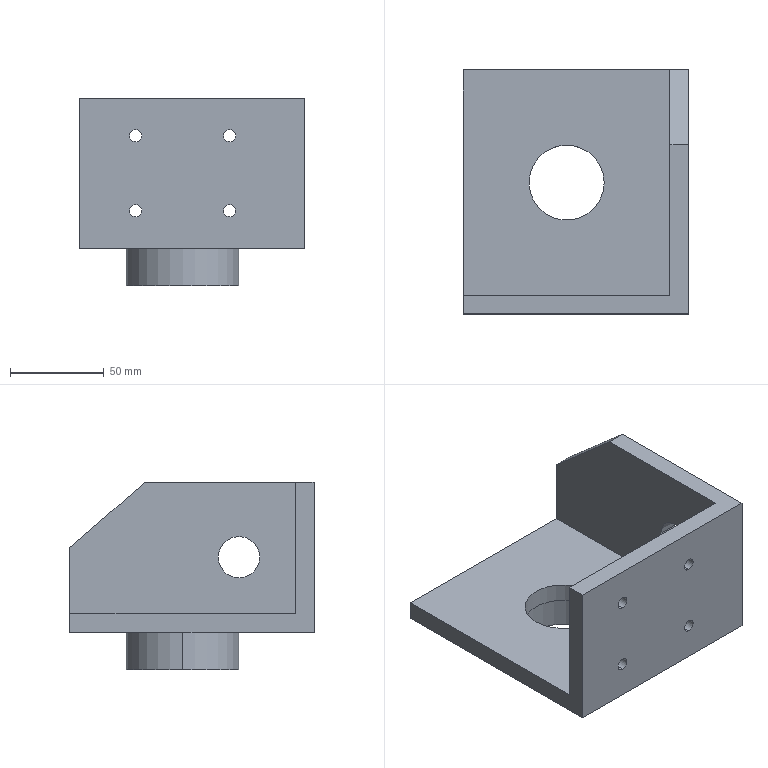Part | NX | features BREP 1 | 1 solid | 28 faces | box 120 x 130 x 100 mm | volume 313379 mm3 | cylinder 16 | plane 12 | commonest cylinder face diameters 6.5 x8 22 x2 40 x2 52 x2 60 x2
STEP:
#1=CARTESIAN_POINT('',(-30.,0.,20.));
#2=VERTEX_POINT('',#1);
#3=CARTESIAN_POINT('',(30.,0.,20.));
#4=VERTEX_POINT('',#3);
#5=CARTESIAN_POINT('',(0.,0.,20.));
#6=DIRECTION('',(0.,0.,-1.));
#7=DIRECTION('',(-1.,0.,0.));
#8=AXIS2_PLACEMENT_3D('',#5,#6,#7);
#9=CIRCLE('',#8,30.);
#10=EDGE_CURVE('',#2,#4,#9,.T.);
#11=ORIENTED_EDGE('',*,*,#10,.T.);
#12=CARTESIAN_POINT('',(30.,0.,0.));
#13=VERTEX_POINT('',#12);
#14=CARTESIAN_POINT('',(30.,0.,20.));
#15=DIRECTION('',(0.,0.,-1.));
#16=VECTOR('',#15,1000.);
#17=LINE('',#14,#16);
#18=EDGE_CURVE('',#4,#13,#17,.T.);
#19=ORIENTED_EDGE('',*,*,#18,.T.);
#20=CARTESIAN_POINT('',(-30.,0.,0.));
#21=VERTEX_POINT('',#20);
#22=CARTESIAN_POINT('',(0.,0.,0.));
#23=DIRECTION('',(0.,0.,1.));
#24=DIRECTION('',(-1.,0.,0.));
#25=AXIS2_PLACEMENT_3D('',#22,#23,#24);
#26=CIRCLE('',#25,30.);
#27=EDGE_CURVE('',#13,#21,#26,.T.);
#28=ORIENTED_EDGE('',*,*,#27,.T.);
#29=CARTESIAN_POINT('',(-30.,0.,20.));
#30=DIRECTION('',(0.,0.,-1.));
#31=VECTOR('',#30,1000.);
#32=LINE('',#29,#31);
#33=EDGE_CURVE('',#2,#21,#32,.T.);
#34=ORIENTED_EDGE('',*,*,#33,.F.);
#35=EDGE_LOOP('',(#11,#19,#28,#34));
#36=FACE_BOUND('',#35,.T.);
#37=CARTESIAN_POINT('',(0.,0.,20.));
#38=DIRECTION('',(0.,0.,-1.));
#39=DIRECTION('',(-1.,0.,0.));
#40=AXIS2_PLACEMENT_3D('',#37,#38,#39);
#41=CYLINDRICAL_SURFACE('',#40,30.);
#42=ADVANCED_FACE('',(#36),#41,.T.);
#43=CARTESIAN_POINT('',(55.,-41.,60.));
#44=VERTEX_POINT('',#43);
#45=CARTESIAN_POINT('',(55.,-19.,60.));
#46=VERTEX_POINT('',#45);
#47=CARTESIAN_POINT('',(55.,-30.,60.));
#48=DIRECTION('',(1.,0.,0.));
#49=DIRECTION('',(0.,1.,0.));
#50=AXIS2_PLACEMENT_3D('',#47,#48,#49);
#51=CIRCLE('',#50,11.);
#52=EDGE_CURVE('',#44,#46,#51,.T.);
#53=ORIENTED_EDGE('',*,*,#52,.F.);
#54=CARTESIAN_POINT('',(65.,-41.,60.));
#55=VERTEX_POINT('',#54);
#56=CARTESIAN_POINT('',(55.,-41.,60.));
#57=DIRECTION('',(1.,0.,0.));
#58=VECTOR('',#57,1000.);
#59=LINE('',#56,#58);
#60=EDGE_CURVE('',#55,#44,#59,.F.);
#61=ORIENTED_EDGE('',*,*,#60,.F.);
#62=CARTESIAN_POINT('',(65.,-19.,60.));
#63=VERTEX_POINT('',#62);
#64=CARTESIAN_POINT('',(65.,-30.,60.));
#65=DIRECTION('',(1.,0.,0.));
#66=DIRECTION('',(0.,1.,0.));
#67=AXIS2_PLACEMENT_3D('',#64,#65,#66);
#68=CIRCLE('',#67,11.);
#69=EDGE_CURVE('',#55,#63,#68,.T.);
#70=ORIENTED_EDGE('',*,*,#69,.T.);
#71=CARTESIAN_POINT('',(55.,-19.,60.));
#72=DIRECTION('',(1.,0.,0.));
#73=VECTOR('',#72,1000.);
#74=LINE('',#71,#73);
#75=EDGE_CURVE('',#63,#46,#74,.F.);
#76=ORIENTED_EDGE('',*,*,#75,.T.);
#77=EDGE_LOOP('',(#53,#61,#70,#76));
#78=FACE_BOUND('',#77,.T.);
#79=CARTESIAN_POINT('',(55.,-30.,60.));
#80=DIRECTION('',(1.,0.,0.));
#81=DIRECTION('',(0.,1.,0.));
#82=AXIS2_PLACEMENT_3D('',#79,#80,#81);
#83=CYLINDRICAL_SURFACE('',#82,11.);
#84=ADVANCED_FACE('',(#78),#83,.F.);
#85=CARTESIAN_POINT('',(-25.,-60.,83.25));
#86=VERTEX_POINT('',#85);
#87=CARTESIAN_POINT('',(-25.,-60.,76.75));
#88=VERTEX_POINT('',#87);
#89=CARTESIAN_POINT('',(-25.,-60.,80.));
#90=DIRECTION('',(0.,-1.,0.));
#91=DIRECTION('',(0.,0.,-1.));
#92=AXIS2_PLACEMENT_3D('',#89,#90,#91);
#93=CIRCLE('',#92,3.25);
#94=EDGE_CURVE('',#86,#88,#93,.T.);
#95=ORIENTED_EDGE('',*,*,#94,.F.);
#96=CARTESIAN_POINT('',(-25.,-70.,83.25));
#97=VERTEX_POINT('',#96);
#98=CARTESIAN_POINT('',(-25.,-60.,83.25));
#99=DIRECTION('',(0.,-1.,0.));
#100=VECTOR('',#99,1000.);
#101=LINE('',#98,#100);
#102=EDGE_CURVE('',#86,#97,#101,.T.);
#103=ORIENTED_EDGE('',*,*,#102,.T.);
#104=CARTESIAN_POINT('',(-25.,-70.,76.75));
#105=VERTEX_POINT('',#104);
#106=CARTESIAN_POINT('',(-25.,-70.,80.));
#107=DIRECTION('',(0.,1.,0.));
#108=DIRECTION('',(0.,0.,-1.));
#109=AXIS2_PLACEMENT_3D('',#106,#107,#108);
#110=CIRCLE('',#109,3.25);
#111=EDGE_CURVE('',#105,#97,#110,.T.);
#112=ORIENTED_EDGE('',*,*,#111,.F.);
#113=CARTESIAN_POINT('',(-25.,-60.,76.75));
#114=DIRECTION('',(0.,-1.,0.));
#115=VECTOR('',#114,1000.);
#116=LINE('',#113,#115);
#117=EDGE_CURVE('',#88,#105,#116,.T.);
#118=ORIENTED_EDGE('',*,*,#117,.F.);
#119=EDGE_LOOP('',(#95,#103,#112,#118));
#120=FACE_BOUND('',#119,.T.);
#121=CARTESIAN_POINT('',(-25.,-60.,80.));
#122=DIRECTION('',(0.,-1.,0.));
#123=DIRECTION('',(0.,0.,-1.));
#124=AXIS2_PLACEMENT_3D('',#121,#122,#123);
#125=CYLINDRICAL_SURFACE('',#124,3.25);
#126=ADVANCED_FACE('',(#120),#125,.F.);
#127=CARTESIAN_POINT('',(25.,-60.,83.25));
#128=VERTEX_POINT('',#127);
#129=CARTESIAN_POINT('',(25.,-60.,76.75));
#130=VERTEX_POINT('',#129);
#131=CARTESIAN_POINT('',(25.,-60.,80.));
#132=DIRECTION('',(0.,-1.,0.));
#133=DIRECTION('',(0.,0.,-1.));
#134=AXIS2_PLACEMENT_3D('',#131,#132,#133);
#135=CIRCLE('',#134,3.25);
#136=EDGE_CURVE('',#128,#130,#135,.T.);
#137=ORIENTED_EDGE('',*,*,#136,.F.);
#138=CARTESIAN_POINT('',(25.,-70.,83.25));
#139=VERTEX_POINT('',#138);
#140=CARTESIAN_POINT('',(25.,-60.,83.25));
#141=DIRECTION('',(0.,-1.,0.));
#142=VECTOR('',#141,1000.);
#143=LINE('',#140,#142);
#144=EDGE_CURVE('',#128,#139,#143,.T.);
#145=ORIENTED_EDGE('',*,*,#144,.T.);
#146=CARTESIAN_POINT('',(25.,-70.,76.75));
#147=VERTEX_POINT('',#146);
#148=CARTESIAN_POINT('',(25.,-70.,80.));
#149=DIRECTION('',(0.,1.,0.));
#150=DIRECTION('',(0.,0.,-1.));
#151=AXIS2_PLACEMENT_3D('',#148,#149,#150);
#152=CIRCLE('',#151,3.25);
#153=EDGE_CURVE('',#147,#139,#152,.T.);
#154=ORIENTED_EDGE('',*,*,#153,.F.);
#155=CARTESIAN_POINT('',(25.,-60.,76.75));
#156=DIRECTION('',(0.,-1.,0.));
#157=VECTOR('',#156,1000.);
#158=LINE('',#155,#157);
#159=EDGE_CURVE('',#130,#147,#158,.T.);
#160=ORIENTED_EDGE('',*,*,#159,.F.);
#161=EDGE_LOOP('',(#137,#145,#154,#160));
#162=FACE_BOUND('',#161,.T.);
#163=CARTESIAN_POINT('',(25.,-60.,80.));
#164=DIRECTION('',(0.,-1.,0.));
#165=DIRECTION('',(0.,0.,-1.));
#166=AXIS2_PLACEMENT_3D('',#163,#164,#165);
#167=CYLINDRICAL_SURFACE('',#166,3.25);
#168=ADVANCED_FACE('',(#162),#167,.F.);
#169=CARTESIAN_POINT('',(25.,-60.,43.25));
#170=VERTEX_POINT('',#169);
#171=CARTESIAN_POINT('',(25.,-60.,36.75));
#172=VERTEX_POINT('',#171);
#173=CARTESIAN_POINT('',(25.,-60.,40.));
#174=DIRECTION('',(0.,-1.,0.));
#175=DIRECTION('',(0.,0.,-1.));
#176=AXIS2_PLACEMENT_3D('',#173,#174,#175);
#177=CIRCLE('',#176,3.25);
#178=EDGE_CURVE('',#170,#172,#177,.T.);
#179=ORIENTED_EDGE('',*,*,#178,.F.);
#180=CARTESIAN_POINT('',(25.,-70.,43.25));
#181=VERTEX_POINT('',#180);
#182=CARTESIAN_POINT('',(25.,-60.,43.25));
#183=DIRECTION('',(0.,-1.,0.));
#184=VECTOR('',#183,1000.);
#185=LINE('',#182,#184);
#186=EDGE_CURVE('',#170,#181,#185,.T.);
#187=ORIENTED_EDGE('',*,*,#186,.T.);
#188=CARTESIAN_POINT('',(25.,-70.,36.75));
#189=VERTEX_POINT('',#188);
#190=CARTESIAN_POINT('',(25.,-70.,40.));
#191=DIRECTION('',(0.,1.,0.));
#192=DIRECTION('',(0.,0.,-1.));
#193=AXIS2_PLACEMENT_3D('',#190,#191,#192);
#194=CIRCLE('',#193,3.25);
#195=EDGE_CURVE('',#189,#181,#194,.T.);
#196=ORIENTED_EDGE('',*,*,#195,.F.);
#197=CARTESIAN_POINT('',(25.,-60.,36.75));
#198=DIRECTION('',(0.,-1.,0.));
#199=VECTOR('',#198,1000.);
#200=LINE('',#197,#199);
#201=EDGE_CURVE('',#172,#189,#200,.T.);
#202=ORIENTED_EDGE('',*,*,#201,.F.);
#203=EDGE_LOOP('',(#179,#187,#196,#202));
#204=FACE_BOUND('',#203,.T.);
#205=CARTESIAN_POINT('',(25.,-60.,40.));
#206=DIRECTION('',(0.,-1.,0.));
#207=DIRECTION('',(0.,0.,-1.));
#208=AXIS2_PLACEMENT_3D('',#205,#206,#207);
#209=CYLINDRICAL_SURFACE('',#208,3.25);
#210=ADVANCED_FACE('',(#204),#209,.F.);
#211=CARTESIAN_POINT('',(-25.,-60.,43.25));
#212=VERTEX_POINT('',#211);
#213=CARTESIAN_POINT('',(-25.,-60.,36.75));
#214=VERTEX_POINT('',#213);
#215=CARTESIAN_POINT('',(-25.,-60.,40.));
#216=DIRECTION('',(0.,-1.,0.));
#217=DIRECTION('',(0.,0.,-1.));
#218=AXIS2_PLACEMENT_3D('',#215,#216,#217);
#219=CIRCLE('',#218,3.25);
#220=EDGE_CURVE('',#212,#214,#219,.T.);
#221=ORIENTED_EDGE('',*,*,#220,.F.);
#222=CARTESIAN_POINT('',(-25.,-70.,43.25));
#223=VERTEX_POINT('',#222);
#224=CARTESIAN_POINT('',(-25.,-60.,43.25));
#225=DIRECTION('',(0.,-1.,0.));
#226=VECTOR('',#225,1000.);
#227=LINE('',#224,#226);
#228=EDGE_CURVE('',#212,#223,#227,.T.);
#229=ORIENTED_EDGE('',*,*,#228,.T.);
#230=CARTESIAN_POINT('',(-25.,-70.,36.75));
#231=VERTEX_POINT('',#230);
#232=CARTESIAN_POINT('',(-25.,-70.,40.));
#233=DIRECTION('',(0.,1.,0.));
#234=DIRECTION('',(0.,0.,-1.));
#235=AXIS2_PLACEMENT_3D('',#232,#233,#234);
#236=CIRCLE('',#235,3.25);
#237=EDGE_CURVE('',#231,#223,#236,.T.);
#238=ORIENTED_EDGE('',*,*,#237,.F.);
#239=CARTESIAN_POINT('',(-25.,-60.,36.75));
#240=DIRECTION('',(0.,-1.,0.));
#241=VECTOR('',#240,1000.);
#242=LINE('',#239,#241);
#243=EDGE_CURVE('',#214,#231,#242,.T.);
#244=ORIENTED_EDGE('',*,*,#243,.F.);
#245=EDGE_LOOP('',(#221,#229,#238,#244));
#246=FACE_BOUND('',#245,.T.);
#247=CARTESIAN_POINT('',(-25.,-60.,40.));
#248=DIRECTION('',(0.,-1.,0.));
#249=DIRECTION('',(0.,0.,-1.));
#250=AXIS2_PLACEMENT_3D('',#247,#248,#249);
#251=CYLINDRICAL_SURFACE('',#250,3.25);
#252=ADVANCED_FACE('',(#246),#251,.F.);
#253=CARTESIAN_POINT('',(26.,0.,20.));
#254=VERTEX_POINT('',#253);
#255=CARTESIAN_POINT('',(-26.,0.,20.));
#256=VERTEX_POINT('',#255);
#257=CARTESIAN_POINT('',(0.,0.,20.));
#258=DIRECTION('',(0.,0.,-1.));
#259=DIRECTION('',(-1.,0.,0.));
#260=AXIS2_PLACEMENT_3D('',#257,#258,#259);
#261=CIRCLE('',#260,26.);
#262=EDGE_CURVE('',#254,#256,#261,.T.);
#263=ORIENTED_EDGE('',*,*,#262,.F.);
#264=CARTESIAN_POINT('',(26.,0.,0.));
#265=VERTEX_POINT('',#264);
#266=CARTESIAN_POINT('',(26.,0.,20.));
#267=DIRECTION('',(0.,0.,-1.));
#268=VECTOR('',#267,1000.);
#269=LINE('',#266,#268);
#270=EDGE_CURVE('',#254,#265,#269,.T.);
#271=ORIENTED_EDGE('',*,*,#270,.T.);
#272=CARTESIAN_POINT('',(-26.,0.,0.));
#273=VERTEX_POINT('',#272);
#274=CARTESIAN_POINT('',(0.,0.,0.));
#275=DIRECTION('',(0.,0.,-1.));
#276=DIRECTION('',(-1.,0.,0.));
#277=AXIS2_PLACEMENT_3D('',#274,#275,#276);
#278=CIRCLE('',#277,26.);
#279=EDGE_CURVE('',#265,#273,#278,.T.);
#280=ORIENTED_EDGE('',*,*,#279,.T.);
#281=CARTESIAN_POINT('',(-26.,0.,20.));
#282=DIRECTION('',(0.,0.,-1.));
#283=VECTOR('',#282,1000.);
#284=LINE('',#281,#283);
#285=EDGE_CURVE('',#256,#273,#284,.T.);
#286=ORIENTED_EDGE('',*,*,#285,.F.);
#287=EDGE_LOOP('',(#263,#271,#280,#286));
#288=FACE_BOUND('',#287,.T.);
#289=CARTESIAN_POINT('',(0.,0.,20.));
#290=DIRECTION('',(0.,0.,-1.));
#291=DIRECTION('',(-1.,0.,0.));
#292=AXIS2_PLACEMENT_3D('',#289,#290,#291);
#293=CYLINDRICAL_SURFACE('',#292,26.);
#294=ADVANCED_FACE('',(#288),#293,.F.);
#295=CARTESIAN_POINT('',(20.,0.,30.));
#296=VERTEX_POINT('',#295);
#297=CARTESIAN_POINT('',(-20.,0.,30.));
#298=VERTEX_POINT('',#297);
#299=CARTESIAN_POINT('',(0.,0.,30.));
#300=DIRECTION('',(0.,0.,-1.));
#301=DIRECTION('',(-1.,0.,0.));
#302=AXIS2_PLACEMENT_3D('',#299,#300,#301);
#303=CIRCLE('',#302,20.);
#304=EDGE_CURVE('',#296,#298,#303,.T.);
#305=ORIENTED_EDGE('',*,*,#304,.F.);
#306=CARTESIAN_POINT('',(20.,0.,20.));
#307=VERTEX_POINT('',#306);
#308=CARTESIAN_POINT('',(20.,0.,30.));
#309=DIRECTION('',(0.,0.,-1.));
#310=VECTOR('',#309,1000.);
#311=LINE('',#308,#310);
#312=EDGE_CURVE('',#296,#307,#311,.T.);
#313=ORIENTED_EDGE('',*,*,#312,.T.);
#314=CARTESIAN_POINT('',(-20.,0.,20.));
#315=VERTEX_POINT('',#314);
#316=CARTESIAN_POINT('',(0.,0.,20.));
#317=DIRECTION('',(0.,0.,1.));
#318=DIRECTION('',(-1.,0.,0.));
#319=AXIS2_PLACEMENT_3D('',#316,#317,#318);
#320=CIRCLE('',#319,20.);
#321=EDGE_CURVE('',#315,#307,#320,.T.);
#322=ORIENTED_EDGE('',*,*,#321,.F.);
#323=CARTESIAN_POINT('',(-20.,0.,30.));
#324=DIRECTION('',(0.,0.,-1.));
#325=VECTOR('',#324,1000.);
#326=LINE('',#323,#325);
#327=EDGE_CURVE('',#298,#315,#326,.T.);
#328=ORIENTED_EDGE('',*,*,#327,.F.);
#329=EDGE_LOOP('',(#305,#313,#322,#328));
#330=FACE_BOUND('',#329,.T.);
#331=CARTESIAN_POINT('',(0.,0.,30.));
#332=DIRECTION('',(0.,0.,-1.));
#333=DIRECTION('',(-1.,0.,0.));
#334=AXIS2_PLACEMENT_3D('',#331,#332,#333);
#335=CYLINDRICAL_SURFACE('',#334,20.);
#336=ADVANCED_FACE('',(#330),#335,.F.);
#337=CARTESIAN_POINT('',(-55.,-70.,20.));
#338=VERTEX_POINT('',#337);
#339=CARTESIAN_POINT('',(65.,-70.,20.));
#340=VERTEX_POINT('',#339);
#341=CARTESIAN_POINT('',(65.,-70.,20.));
#342=DIRECTION('',(1.,0.,0.));
#343=VECTOR('',#342,1000.);
#344=LINE('',#341,#343);
#345=EDGE_CURVE('',#338,#340,#344,.T.);
#346=ORIENTED_EDGE('',*,*,#345,.F.);
#347=CARTESIAN_POINT('',(-55.,60.,20.));
#348=VERTEX_POINT('',#347);
#349=CARTESIAN_POINT('',(-55.,-60.,20.));
#350=DIRECTION('',(0.,-1.,0.));
#351=VECTOR('',#350,1000.);
#352=LINE('',#349,#351);
#353=EDGE_CURVE('',#348,#338,#352,.T.);
#354=ORIENTED_EDGE('',*,*,#353,.F.);
#355=CARTESIAN_POINT('',(65.,60.,20.));
#356=VERTEX_POINT('',#355);
#357=CARTESIAN_POINT('',(65.,60.,20.));
#358=DIRECTION('',(-1.,0.,0.));
#359=VECTOR('',#358,1000.);
#360=LINE('',#357,#359);
#361=EDGE_CURVE('',#356,#348,#360,.T.);
#362=ORIENTED_EDGE('',*,*,#361,.F.);
#363=CARTESIAN_POINT('',(65.,-60.,20.));
#364=DIRECTION('',(0.,1.,0.));
#365=VECTOR('',#364,1000.);
#366=LINE('',#363,#365);
#367=EDGE_CURVE('',#340,#356,#366,.T.);
#368=ORIENTED_EDGE('',*,*,#367,.F.);
#369=EDGE_LOOP('',(#346,#354,#362,#368));
#370=FACE_BOUND('',#369,.T.);
#371=ORIENTED_EDGE('',*,*,#10,.F.);
#372=CARTESIAN_POINT('',(0.,0.,20.));
#373=DIRECTION('',(0.,0.,-1.));
#374=DIRECTION('',(-1.,0.,0.));
#375=AXIS2_PLACEMENT_3D('',#372,#373,#374);
#376=CIRCLE('',#375,30.);
#377=EDGE_CURVE('',#4,#2,#376,.T.);
#378=ORIENTED_EDGE('',*,*,#377,.F.);
#379=EDGE_LOOP('',(#371,#378));
#380=FACE_BOUND('',#379,.T.);
#381=CARTESIAN_POINT('',(65.,-60.,20.));
#382=DIRECTION('',(0.,0.,1.));
#383=DIRECTION('',(1.,0.,0.));
#384=AXIS2_PLACEMENT_3D('',#381,#382,#383);
#385=PLANE('',#384);
#386=ADVANCED_FACE('',(#370,#380),#385,.F.);
#387=ORIENTED_EDGE('',*,*,#18,.F.);
#388=ORIENTED_EDGE('',*,*,#377,.T.);
#389=ORIENTED_EDGE('',*,*,#33,.T.);
#390=CARTESIAN_POINT('',(0.,0.,0.));
#391=DIRECTION('',(0.,0.,1.));
#392=DIRECTION('',(-1.,0.,0.));
#393=AXIS2_PLACEMENT_3D('',#390,#391,#392);
#394=CIRCLE('',#393,30.);
#395=EDGE_CURVE('',#21,#13,#394,.T.);
#396=ORIENTED_EDGE('',*,*,#395,.T.);
#397=EDGE_LOOP('',(#387,#388,#389,#396));
#398=FACE_BOUND('',#397,.T.);
#399=CARTESIAN_POINT('',(0.,0.,20.));
#400=DIRECTION('',(0.,0.,-1.));
#401=DIRECTION('',(-1.,0.,0.));
#402=AXIS2_PLACEMENT_3D('',#399,#400,#401);
#403=CYLINDRICAL_SURFACE('',#402,30.);
#404=ADVANCED_FACE('',(#398),#403,.T.);
#405=CARTESIAN_POINT('',(65.,20.,100.));
#406=VERTEX_POINT('',#405);
#407=CARTESIAN_POINT('',(65.,60.,65.));
#408=VERTEX_POINT('',#407);
#409=CARTESIAN_POINT('',(65.,20.,100.));
#410=DIRECTION('',(0.,0.7526,-0.6585));
#411=VECTOR('',#410,1000.);
#412=LINE('',#409,#411);
#413=EDGE_CURVE('',#406,#408,#412,.T.);
#414=ORIENTED_EDGE('',*,*,#413,.F.);
#415=CARTESIAN_POINT('',(65.,-70.,100.));
#416=VERTEX_POINT('',#415);
#417=CARTESIAN_POINT('',(65.,60.,100.));
#418=DIRECTION('',(0.,1.,0.));
#419=VECTOR('',#418,1000.);
#420=LINE('',#417,#419);
#421=EDGE_CURVE('',#416,#406,#420,.T.);
#422=ORIENTED_EDGE('',*,*,#421,.F.);
#423=CARTESIAN_POINT('',(65.,-70.,30.));
#424=DIRECTION('',(0.,0.,1.));
#425=VECTOR('',#424,1000.);
#426=LINE('',#423,#425);
#427=EDGE_CURVE('',#340,#416,#426,.T.);
#428=ORIENTED_EDGE('',*,*,#427,.F.);
#429=ORIENTED_EDGE('',*,*,#367,.T.);
#430=CARTESIAN_POINT('',(65.,60.,30.));
#431=DIRECTION('',(0.,0.,-1.));
#432=VECTOR('',#431,1000.);
#433=LINE('',#430,#432);
#434=EDGE_CURVE('',#408,#356,#433,.T.);
#435=ORIENTED_EDGE('',*,*,#434,.F.);
#436=EDGE_LOOP('',(#414,#422,#428,#429,#435));
#437=FACE_BOUND('',#436,.T.);
#438=CARTESIAN_POINT('',(65.,-30.,60.));
#439=DIRECTION('',(1.,0.,0.));
#440=DIRECTION('',(0.,1.,0.));
#441=AXIS2_PLACEMENT_3D('',#438,#439,#440);
#442=CIRCLE('',#441,11.);
#443=EDGE_CURVE('',#63,#55,#442,.T.);
#444=ORIENTED_EDGE('',*,*,#443,.F.);
#445=ORIENTED_EDGE('',*,*,#69,.F.);
#446=EDGE_LOOP('',(#444,#445));
#447=FACE_BOUND('',#446,.T.);
#448=CARTESIAN_POINT('',(65.,60.,30.));
#449=DIRECTION('',(-1.,0.,0.));
#450=DIRECTION('',(0.,1.,0.));
#451=AXIS2_PLACEMENT_3D('',#448,#449,#450);
#452=PLANE('',#451);
#453=ADVANCED_FACE('',(#437,#447),#452,.F.);
#454=ORIENTED_EDGE('',*,*,#427,.T.);
#455=CARTESIAN_POINT('',(-55.,-70.,100.));
#456=VERTEX_POINT('',#455);
#457=CARTESIAN_POINT('',(-135.623,-70.,100.));
#458=DIRECTION('',(-1.,0.,0.));
#459=VECTOR('',#458,1000.);
#460=LINE('',#457,#459);
#461=EDGE_CURVE('',#416,#456,#460,.T.);
#462=ORIENTED_EDGE('',*,*,#461,.T.);
#463=CARTESIAN_POINT('',(-55.,-70.,100.));
#464=DIRECTION('',(0.,0.,-1.));
#465=VECTOR('',#464,1000.);
#466=LINE('',#463,#465);
#467=EDGE_CURVE('',#456,#338,#466,.T.);
#468=ORIENTED_EDGE('',*,*,#467,.T.);
#469=ORIENTED_EDGE('',*,*,#345,.T.);
#470=EDGE_LOOP('',(#454,#462,#468,#469));
#471=FACE_BOUND('',#470,.T.);
#472=ORIENTED_EDGE('',*,*,#111,.T.);
#473=CARTESIAN_POINT('',(-25.,-70.,80.));
#474=DIRECTION('',(0.,1.,0.));
#475=DIRECTION('',(0.,0.,-1.));
#476=AXIS2_PLACEMENT_3D('',#473,#474,#475);
#477=CIRCLE('',#476,3.25);
#478=EDGE_CURVE('',#97,#105,#477,.T.);
#479=ORIENTED_EDGE('',*,*,#478,.T.);
#480=EDGE_LOOP('',(#472,#479));
#481=FACE_BOUND('',#480,.T.);
#482=ORIENTED_EDGE('',*,*,#153,.T.);
#483=CARTESIAN_POINT('',(25.,-70.,80.));
#484=DIRECTION('',(0.,1.,0.));
#485=DIRECTION('',(0.,0.,-1.));
#486=AXIS2_PLACEMENT_3D('',#483,#484,#485);
#487=CIRCLE('',#486,3.25);
#488=EDGE_CURVE('',#139,#147,#487,.T.);
#489=ORIENTED_EDGE('',*,*,#488,.T.);
#490=EDGE_LOOP('',(#482,#489));
#491=FACE_BOUND('',#490,.T.);
#492=ORIENTED_EDGE('',*,*,#195,.T.);
#493=CARTESIAN_POINT('',(25.,-70.,40.));
#494=DIRECTION('',(0.,1.,0.));
#495=DIRECTION('',(0.,0.,-1.));
#496=AXIS2_PLACEMENT_3D('',#493,#494,#495);
#497=CIRCLE('',#496,3.25);
#498=EDGE_CURVE('',#181,#189,#497,.T.);
#499=ORIENTED_EDGE('',*,*,#498,.T.);
#500=EDGE_LOOP('',(#492,#499));
#501=FACE_BOUND('',#500,.T.);
#502=ORIENTED_EDGE('',*,*,#237,.T.);
#503=CARTESIAN_POINT('',(-25.,-70.,40.));
#504=DIRECTION('',(0.,1.,0.));
#505=DIRECTION('',(0.,0.,-1.));
#506=AXIS2_PLACEMENT_3D('',#503,#504,#505);
#507=CIRCLE('',#506,3.25);
#508=EDGE_CURVE('',#223,#231,#507,.T.);
#509=ORIENTED_EDGE('',*,*,#508,.T.);
#510=EDGE_LOOP('',(#502,#509));
#511=FACE_BOUND('',#510,.T.);
#512=CARTESIAN_POINT('',(-135.623,-70.,100.));
#513=DIRECTION('',(0.,-1.,0.));
#514=DIRECTION('',(0.,0.,-1.));
#515=AXIS2_PLACEMENT_3D('',#512,#513,#514);
#516=PLANE('',#515);
#517=ADVANCED_FACE('',(#471,#481,#491,#501,#511),#516,.T.);
#518=ORIENTED_EDGE('',*,*,#467,.F.);
#519=CARTESIAN_POINT('',(-55.,-60.,100.));
#520=VERTEX_POINT('',#519);
#521=CARTESIAN_POINT('',(-55.,60.,100.));
#522=DIRECTION('',(0.,-1.,0.));
#523=VECTOR('',#522,1000.);
#524=LINE('',#521,#523);
#525=EDGE_CURVE('',#520,#456,#524,.T.);
#526=ORIENTED_EDGE('',*,*,#525,.F.);
#527=CARTESIAN_POINT('',(-55.,-60.,30.));
#528=VERTEX_POINT('',#527);
#529=CARTESIAN_POINT('',(-55.,-60.,30.));
#530=DIRECTION('',(0.,0.,1.));
#531=VECTOR('',#530,1000.);
#532=LINE('',#529,#531);
#533=EDGE_CURVE('',#528,#520,#532,.T.);
#534=ORIENTED_EDGE('',*,*,#533,.F.);
#535=CARTESIAN_POINT('',(-55.,60.,30.));
#536=VERTEX_POINT('',#535);
#537=CARTESIAN_POINT('',(-55.,60.,30.));
#538=DIRECTION('',(0.,-1.,0.));
#539=VECTOR('',#538,1000.);
#540=LINE('',#537,#539);
#541=EDGE_CURVE('',#536,#528,#540,.T.);
#542=ORIENTED_EDGE('',*,*,#541,.F.);
#543=CARTESIAN_POINT('',(-55.,60.,30.));
#544=DIRECTION('',(0.,0.,1.));
#545=VECTOR('',#544,1000.);
#546=LINE('',#543,#545);
#547=EDGE_CURVE('',#348,#536,#546,.T.);
#548=ORIENTED_EDGE('',*,*,#547,.F.);
#549=ORIENTED_EDGE('',*,*,#353,.T.);
#550=EDGE_LOOP('',(#518,#526,#534,#542,#548,#549));
#551=FACE_BOUND('',#550,.T.);
#552=CARTESIAN_POINT('',(-55.,60.,30.));
#553=DIRECTION('',(1.,0.,0.));
#554=DIRECTION('',(0.,1.,0.));
#555=AXIS2_PLACEMENT_3D('',#552,#553,#554);
#556=PLANE('',#555);
#557=ADVANCED_FACE('',(#551),#556,.F.);
#558=ORIENTED_EDGE('',*,*,#547,.T.);
#559=CARTESIAN_POINT('',(55.,60.,30.));
#560=VERTEX_POINT('',#559);
#561=CARTESIAN_POINT('',(-55.,60.,30.));
#562=DIRECTION('',(-1.,0.,0.));
#563=VECTOR('',#562,1000.);
#564=LINE('',#561,#563);
#565=EDGE_CURVE('',#560,#536,#564,.T.);
#566=ORIENTED_EDGE('',*,*,#565,.F.);
#567=CARTESIAN_POINT('',(55.,60.,65.));
#568=VERTEX_POINT('',#567);
#569=CARTESIAN_POINT('',(55.,60.,30.));
#570=DIRECTION('',(0.,0.,-1.));
#571=VECTOR('',#570,1000.);
#572=LINE('',#569,#571);
#573=EDGE_CURVE('',#568,#560,#572,.T.);
#574=ORIENTED_EDGE('',*,*,#573,.F.);
#575=CARTESIAN_POINT('',(-55.,60.,65.));
#576=DIRECTION('',(-1.,0.,0.));
#577=VECTOR('',#576,1000.);
#578=LINE('',#575,#577);
#579=EDGE_CURVE('',#408,#568,#578,.T.);
#580=ORIENTED_EDGE('',*,*,#579,.F.);
#581=ORIENTED_EDGE('',*,*,#434,.T.);
#582=ORIENTED_EDGE('',*,*,#361,.T.);
#583=EDGE_LOOP('',(#558,#566,#574,#580,#581,#582));
#584=FACE_BOUND('',#583,.T.);
#585=CARTESIAN_POINT('',(-55.,60.,30.));
#586=DIRECTION('',(0.,-1.,0.));
#587=DIRECTION('',(0.,0.,-1.));
#588=AXIS2_PLACEMENT_3D('',#585,#586,#587);
#589=PLANE('',#588);
#590=ADVANCED_FACE('',(#584),#589,.F.);
#591=ORIENTED_EDGE('',*,*,#395,.F.);
#592=ORIENTED_EDGE('',*,*,#27,.F.);
#593=EDGE_LOOP('',(#591,#592));
#594=FACE_BOUND('',#593,.T.);
#595=CARTESIAN_POINT('',(0.,0.,0.));
#596=DIRECTION('',(0.,0.,-1.));
#597=DIRECTION('',(-1.,0.,0.));
#598=AXIS2_PLACEMENT_3D('',#595,#596,#597);
#599=CIRCLE('',#598,26.);
#600=EDGE_CURVE('',#273,#265,#599,.T.);
#601=ORIENTED_EDGE('',*,*,#600,.F.);
#602=ORIENTED_EDGE('',*,*,#279,.F.);
#603=EDGE_LOOP('',(#601,#602));
#604=FACE_BOUND('',#603,.T.);
#605=CARTESIAN_POINT('',(0.,0.,0.));
#606=DIRECTION('',(0.,0.,1.));
#607=DIRECTION('',(1.,0.,0.));
#608=AXIS2_PLACEMENT_3D('',#605,#606,#607);
#609=PLANE('',#608);
#610=ADVANCED_FACE('',(#594,#604),#609,.F.);
#611=ORIENTED_EDGE('',*,*,#60,.T.);
#612=CARTESIAN_POINT('',(55.,-30.,60.));
#613=DIRECTION('',(1.,0.,0.));
#614=DIRECTION('',(0.,1.,0.));
#615=AXIS2_PLACEMENT_3D('',#612,#613,#614);
#616=CIRCLE('',#615,11.);
#617=EDGE_CURVE('',#46,#44,#616,.T.);
#618=ORIENTED_EDGE('',*,*,#617,.F.);
#619=ORIENTED_EDGE('',*,*,#75,.F.);
#620=ORIENTED_EDGE('',*,*,#443,.T.);
#621=EDGE_LOOP('',(#611,#618,#619,#620));
#622=FACE_BOUND('',#621,.T.);
#623=CARTESIAN_POINT('',(55.,-30.,60.));
#624=DIRECTION('',(1.,0.,0.));
#625=DIRECTION('',(0.,1.,0.));
#626=AXIS2_PLACEMENT_3D('',#623,#624,#625);
#627=CYLINDRICAL_SURFACE('',#626,11.);
#628=ADVANCED_FACE('',(#622),#627,.F.);
#629=CARTESIAN_POINT('',(55.,20.,100.));
#630=VERTEX_POINT('',#629);
#631=CARTESIAN_POINT('',(55.,20.,100.));
#632=DIRECTION('',(0.,-0.7526,0.6585));
#633=VECTOR('',#632,1000.);
#634=LINE('',#631,#633);
#635=EDGE_CURVE('',#568,#630,#634,.T.);
#636=ORIENTED_EDGE('',*,*,#635,.T.);
#637=CARTESIAN_POINT('',(55.,20.,100.));
#638=DIRECTION('',(1.,0.,0.));
#639=VECTOR('',#638,1000.);
#640=LINE('',#637,#639);
#641=EDGE_CURVE('',#630,#406,#640,.T.);
#642=ORIENTED_EDGE('',*,*,#641,.T.);
#643=ORIENTED_EDGE('',*,*,#413,.T.);
#644=ORIENTED_EDGE('',*,*,#579,.T.);
#645=EDGE_LOOP('',(#636,#642,#643,#644));
#646=FACE_BOUND('',#645,.T.);
#647=CARTESIAN_POINT('',(55.,20.,100.));
#648=DIRECTION('',(0.,0.6585,0.7526));
#649=DIRECTION('',(1.,0.,0.));
#650=AXIS2_PLACEMENT_3D('',#647,#648,#649);
#651=PLANE('',#650);
#652=ADVANCED_FACE('',(#646),#651,.T.);
#653=CARTESIAN_POINT('',(55.,-60.,100.));
#654=VERTEX_POINT('',#653);
#655=CARTESIAN_POINT('',(55.,-60.,100.));
#656=DIRECTION('',(0.,-1.,0.));
#657=VECTOR('',#656,1000.);
#658=LINE('',#655,#657);
#659=EDGE_CURVE('',#630,#654,#658,.T.);
#660=ORIENTED_EDGE('',*,*,#659,.T.);
#661=CARTESIAN_POINT('',(-135.623,-60.,100.));
#662=DIRECTION('',(-1.,0.,0.));
#663=VECTOR('',#662,1000.);
#664=LINE('',#661,#663);
#665=EDGE_CURVE('',#654,#520,#664,.T.);
#666=ORIENTED_EDGE('',*,*,#665,.T.);
#667=ORIENTED_EDGE('',*,*,#525,.T.);
#668=ORIENTED_EDGE('',*,*,#461,.F.);
#669=ORIENTED_EDGE('',*,*,#421,.T.);
#670=ORIENTED_EDGE('',*,*,#641,.F.);
#671=EDGE_LOOP('',(#660,#666,#667,#668,#669,#670));
#672=FACE_BOUND('',#671,.T.);
#673=CARTESIAN_POINT('',(-135.623,-60.,100.));
#674=DIRECTION('',(0.,0.,1.));
#675=DIRECTION('',(1.,0.,0.));
#676=AXIS2_PLACEMENT_3D('',#673,#674,#675);
#677=PLANE('',#676);
#678=ADVANCED_FACE('',(#672),#677,.T.);
#679=ORIENTED_EDGE('',*,*,#102,.F.);
#680=CARTESIAN_POINT('',(-25.,-60.,80.));
#681=DIRECTION('',(0.,-1.,0.));
#682=DIRECTION('',(0.,0.,-1.));
#683=AXIS2_PLACEMENT_3D('',#680,#681,#682);
#684=CIRCLE('',#683,3.25);
#685=EDGE_CURVE('',#88,#86,#684,.T.);
#686=ORIENTED_EDGE('',*,*,#685,.F.);
#687=ORIENTED_EDGE('',*,*,#117,.T.);
#688=ORIENTED_EDGE('',*,*,#478,.F.);
#689=EDGE_LOOP('',(#679,#686,#687,#688));
#690=FACE_BOUND('',#689,.T.);
#691=CARTESIAN_POINT('',(-25.,-60.,80.));
#692=DIRECTION('',(0.,-1.,0.));
#693=DIRECTION('',(0.,0.,-1.));
#694=AXIS2_PLACEMENT_3D('',#691,#692,#693);
#695=CYLINDRICAL_SURFACE('',#694,3.25);
#696=ADVANCED_FACE('',(#690),#695,.F.);
#697=ORIENTED_EDGE('',*,*,#144,.F.);
#698=CARTESIAN_POINT('',(25.,-60.,80.));
#699=DIRECTION('',(0.,-1.,0.));
#700=DIRECTION('',(0.,0.,-1.));
#701=AXIS2_PLACEMENT_3D('',#698,#699,#700);
#702=CIRCLE('',#701,3.25);
#703=EDGE_CURVE('',#130,#128,#702,.T.);
#704=ORIENTED_EDGE('',*,*,#703,.F.);
#705=ORIENTED_EDGE('',*,*,#159,.T.);
#706=ORIENTED_EDGE('',*,*,#488,.F.);
#707=EDGE_LOOP('',(#697,#704,#705,#706));
#708=FACE_BOUND('',#707,.T.);
#709=CARTESIAN_POINT('',(25.,-60.,80.));
#710=DIRECTION('',(0.,-1.,0.));
#711=DIRECTION('',(0.,0.,-1.));
#712=AXIS2_PLACEMENT_3D('',#709,#710,#711);
#713=CYLINDRICAL_SURFACE('',#712,3.25);
#714=ADVANCED_FACE('',(#708),#713,.F.);
#715=ORIENTED_EDGE('',*,*,#186,.F.);
#716=CARTESIAN_POINT('',(25.,-60.,40.));
#717=DIRECTION('',(0.,-1.,0.));
#718=DIRECTION('',(0.,0.,-1.));
#719=AXIS2_PLACEMENT_3D('',#716,#717,#718);
#720=CIRCLE('',#719,3.25);
#721=EDGE_CURVE('',#172,#170,#720,.T.);
#722=ORIENTED_EDGE('',*,*,#721,.F.);
#723=ORIENTED_EDGE('',*,*,#201,.T.);
#724=ORIENTED_EDGE('',*,*,#498,.F.);
#725=EDGE_LOOP('',(#715,#722,#723,#724));
#726=FACE_BOUND('',#725,.T.);
#727=CARTESIAN_POINT('',(25.,-60.,40.));
#728=DIRECTION('',(0.,-1.,0.));
#729=DIRECTION('',(0.,0.,-1.));
#730=AXIS2_PLACEMENT_3D('',#727,#728,#729);
#731=CYLINDRICAL_SURFACE('',#730,3.25);
#732=ADVANCED_FACE('',(#726),#731,.F.);
#733=ORIENTED_EDGE('',*,*,#228,.F.);
#734=CARTESIAN_POINT('',(-25.,-60.,40.));
#735=DIRECTION('',(0.,-1.,0.));
#736=DIRECTION('',(0.,0.,-1.));
#737=AXIS2_PLACEMENT_3D('',#734,#735,#736);
#738=CIRCLE('',#737,3.25);
#739=EDGE_CURVE('',#214,#212,#738,.T.);
#740=ORIENTED_EDGE('',*,*,#739,.F.);
#741=ORIENTED_EDGE('',*,*,#243,.T.);
#742=ORIENTED_EDGE('',*,*,#508,.F.);
#743=EDGE_LOOP('',(#733,#740,#741,#742));
#744=FACE_BOUND('',#743,.T.);
#745=CARTESIAN_POINT('',(-25.,-60.,40.));
#746=DIRECTION('',(0.,-1.,0.));
#747=DIRECTION('',(0.,0.,-1.));
#748=AXIS2_PLACEMENT_3D('',#745,#746,#747);
#749=CYLINDRICAL_SURFACE('',#748,3.25);
#750=ADVANCED_FACE('',(#744),#749,.F.);
#751=ORIENTED_EDGE('',*,*,#533,.T.);
#752=ORIENTED_EDGE('',*,*,#665,.F.);
#753=CARTESIAN_POINT('',(55.,-60.,30.));
#754=VERTEX_POINT('',#753);
#755=CARTESIAN_POINT('',(55.,-60.,100.));
#756=DIRECTION('',(0.,0.,-1.));
#757=VECTOR('',#756,1000.);
#758=LINE('',#755,#757);
#759=EDGE_CURVE('',#654,#754,#758,.T.);
#760=ORIENTED_EDGE('',*,*,#759,.T.);
#761=CARTESIAN_POINT('',(-135.623,-60.,30.));
#762=DIRECTION('',(-1.,0.,0.));
#763=VECTOR('',#762,1000.);
#764=LINE('',#761,#763);
#765=EDGE_CURVE('',#754,#528,#764,.T.);
#766=ORIENTED_EDGE('',*,*,#765,.T.);
#767=EDGE_LOOP('',(#751,#752,#760,#766));
#768=FACE_BOUND('',#767,.T.);
#769=ORIENTED_EDGE('',*,*,#685,.T.);
#770=ORIENTED_EDGE('',*,*,#94,.T.);
#771=EDGE_LOOP('',(#769,#770));
#772=FACE_BOUND('',#771,.T.);
#773=ORIENTED_EDGE('',*,*,#703,.T.);
#774=ORIENTED_EDGE('',*,*,#136,.T.);
#775=EDGE_LOOP('',(#773,#774));
#776=FACE_BOUND('',#775,.T.);
#777=ORIENTED_EDGE('',*,*,#721,.T.);
#778=ORIENTED_EDGE('',*,*,#178,.T.);
#779=EDGE_LOOP('',(#777,#778));
#780=FACE_BOUND('',#779,.T.);
#781=ORIENTED_EDGE('',*,*,#739,.T.);
#782=ORIENTED_EDGE('',*,*,#220,.T.);
#783=EDGE_LOOP('',(#781,#782));
#784=FACE_BOUND('',#783,.T.);
#785=CARTESIAN_POINT('',(-135.623,-60.,100.));
#786=DIRECTION('',(0.,1.,0.));
#787=DIRECTION('',(1.,0.,0.));
#788=AXIS2_PLACEMENT_3D('',#785,#786,#787);
#789=PLANE('',#788);
#790=ADVANCED_FACE('',(#768,#772,#776,#780,#784),#789,.T.);
#791=ORIENTED_EDGE('',*,*,#541,.T.);
#792=ORIENTED_EDGE('',*,*,#765,.F.);
#793=CARTESIAN_POINT('',(55.,-60.,30.));
#794=DIRECTION('',(0.,1.,0.));
#795=VECTOR('',#794,1000.);
#796=LINE('',#793,#795);
#797=EDGE_CURVE('',#754,#560,#796,.T.);
#798=ORIENTED_EDGE('',*,*,#797,.T.);
#799=ORIENTED_EDGE('',*,*,#565,.T.);
#800=EDGE_LOOP('',(#791,#792,#798,#799));
#801=FACE_BOUND('',#800,.T.);
#802=CARTESIAN_POINT('',(0.,0.,30.));
#803=DIRECTION('',(0.,0.,-1.));
#804=DIRECTION('',(-1.,0.,0.));
#805=AXIS2_PLACEMENT_3D('',#802,#803,#804);
#806=CIRCLE('',#805,20.);
#807=EDGE_CURVE('',#298,#296,#806,.T.);
#808=ORIENTED_EDGE('',*,*,#807,.T.);
#809=ORIENTED_EDGE('',*,*,#304,.T.);
#810=EDGE_LOOP('',(#808,#809));
#811=FACE_BOUND('',#810,.T.);
#812=CARTESIAN_POINT('',(65.,-60.,30.));
#813=DIRECTION('',(0.,0.,1.));
#814=DIRECTION('',(1.,0.,0.));
#815=AXIS2_PLACEMENT_3D('',#812,#813,#814);
#816=PLANE('',#815);
#817=ADVANCED_FACE('',(#801,#811),#816,.T.);
#818=ORIENTED_EDGE('',*,*,#659,.F.);
#819=ORIENTED_EDGE('',*,*,#635,.F.);
#820=ORIENTED_EDGE('',*,*,#573,.T.);
#821=ORIENTED_EDGE('',*,*,#797,.F.);
#822=ORIENTED_EDGE('',*,*,#759,.F.);
#823=EDGE_LOOP('',(#818,#819,#820,#821,#822));
#824=FACE_BOUND('',#823,.T.);
#825=ORIENTED_EDGE('',*,*,#617,.T.);
#826=ORIENTED_EDGE('',*,*,#52,.T.);
#827=EDGE_LOOP('',(#825,#826));
#828=FACE_BOUND('',#827,.T.);
#829=CARTESIAN_POINT('',(55.,60.,30.));
#830=DIRECTION('',(-1.,0.,0.));
#831=DIRECTION('',(0.,0.,1.));
#832=AXIS2_PLACEMENT_3D('',#829,#830,#831);
#833=PLANE('',#832);
#834=ADVANCED_FACE('',(#824,#828),#833,.T.);
#835=ORIENTED_EDGE('',*,*,#270,.F.);
#836=CARTESIAN_POINT('',(0.,0.,20.));
#837=DIRECTION('',(0.,0.,-1.));
#838=DIRECTION('',(-1.,0.,0.));
#839=AXIS2_PLACEMENT_3D('',#836,#837,#838);
#840=CIRCLE('',#839,26.);
#841=EDGE_CURVE('',#256,#254,#840,.T.);
#842=ORIENTED_EDGE('',*,*,#841,.F.);
#843=ORIENTED_EDGE('',*,*,#285,.T.);
#844=ORIENTED_EDGE('',*,*,#600,.T.);
#845=EDGE_LOOP('',(#835,#842,#843,#844));
#846=FACE_BOUND('',#845,.T.);
#847=CARTESIAN_POINT('',(0.,0.,20.));
#848=DIRECTION('',(0.,0.,-1.));
#849=DIRECTION('',(-1.,0.,0.));
#850=AXIS2_PLACEMENT_3D('',#847,#848,#849);
#851=CYLINDRICAL_SURFACE('',#850,26.);
#852=ADVANCED_FACE('',(#846),#851,.F.);
#853=ORIENTED_EDGE('',*,*,#312,.F.);
#854=ORIENTED_EDGE('',*,*,#807,.F.);
#855=ORIENTED_EDGE('',*,*,#327,.T.);
#856=CARTESIAN_POINT('',(0.,0.,20.));
#857=DIRECTION('',(0.,0.,1.));
#858=DIRECTION('',(-1.,0.,0.));
#859=AXIS2_PLACEMENT_3D('',#856,#857,#858);
#860=CIRCLE('',#859,20.);
#861=EDGE_CURVE('',#307,#315,#860,.T.);
#862=ORIENTED_EDGE('',*,*,#861,.F.);
#863=EDGE_LOOP('',(#853,#854,#855,#862));
#864=FACE_BOUND('',#863,.T.);
#865=CARTESIAN_POINT('',(0.,0.,30.));
#866=DIRECTION('',(0.,0.,-1.));
#867=DIRECTION('',(-1.,0.,0.));
#868=AXIS2_PLACEMENT_3D('',#865,#866,#867);
#869=CYLINDRICAL_SURFACE('',#868,20.);
#870=ADVANCED_FACE('',(#864),#869,.F.);
#871=ORIENTED_EDGE('',*,*,#841,.T.);
#872=ORIENTED_EDGE('',*,*,#262,.T.);
#873=EDGE_LOOP('',(#871,#872));
#874=FACE_BOUND('',#873,.T.);
#875=ORIENTED_EDGE('',*,*,#321,.T.);
#876=ORIENTED_EDGE('',*,*,#861,.T.);
#877=EDGE_LOOP('',(#875,#876));
#878=FACE_BOUND('',#877,.T.);
#879=CARTESIAN_POINT('',(65.,-60.,20.));
#880=DIRECTION('',(0.,0.,1.));
#881=DIRECTION('',(1.,0.,0.));
#882=AXIS2_PLACEMENT_3D('',#879,#880,#881);
#883=PLANE('',#882);
#884=ADVANCED_FACE('',(#874,#878),#883,.F.);
#885=CLOSED_SHELL('',(#42,#84,#126,#168,#210,#252,#294,#336,#386,#404,#453,#517,#557,#590,#610,#628,#652,#678,#696,#714,#732,#750,#790,#817,#834,#852,#870,#884));
#886=MANIFOLD_SOLID_BREP('',#885);
#887=(LENGTH_UNIT()NAMED_UNIT(*)SI_UNIT(.MILLI.,.METRE.));
#888=UNCERTAINTY_MEASURE_WITH_UNIT(LENGTH_MEASURE(0.00001),#887,'','');
#889=(NAMED_UNIT(*)PLANE_ANGLE_UNIT()SI_UNIT($,.RADIAN.));
#890=(NAMED_UNIT(*)SI_UNIT($,.STERADIAN.)SOLID_ANGLE_UNIT());
#891=(GEOMETRIC_REPRESENTATION_CONTEXT(3)GLOBAL_UNCERTAINTY_ASSIGNED_CONTEXT((#888))GLOBAL_UNIT_ASSIGNED_CONTEXT((#887,#889,#890))REPRESENTATION_CONTEXT('',''));
#892=ADVANCED_BREP_SHAPE_REPRESENTATION('',(#886),#891);